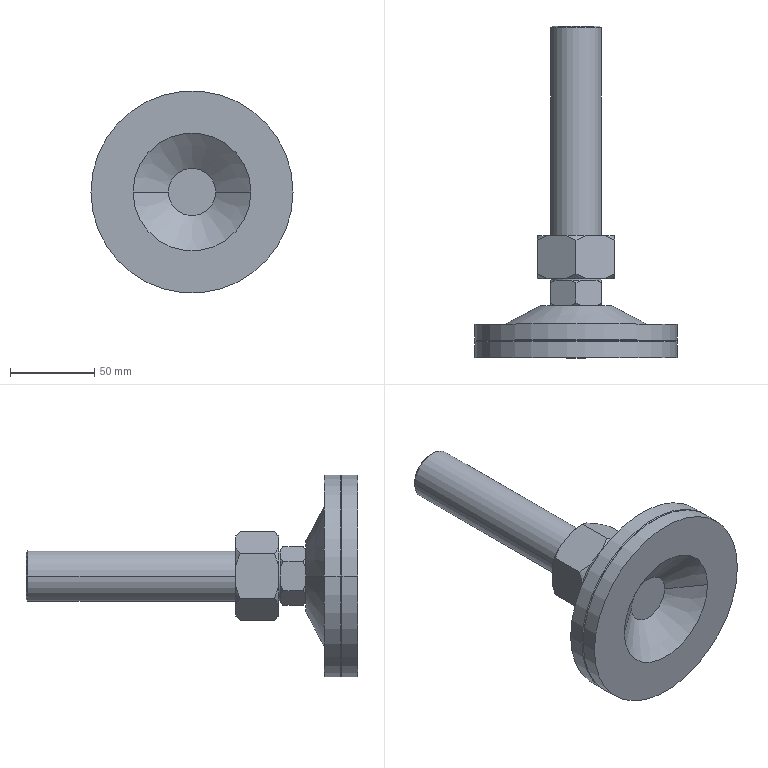Part | SolidWorks | features ICE 2, RevCut 2, Chamfer 1, Revolution 1 | 1 solid | 67 faces | box 120 x 197 x 120 mm | volume 378664 mm3 | cone 34 | plane 25 | cylinder 8 | commonest cylinder face diameters 30 x4 120 x4